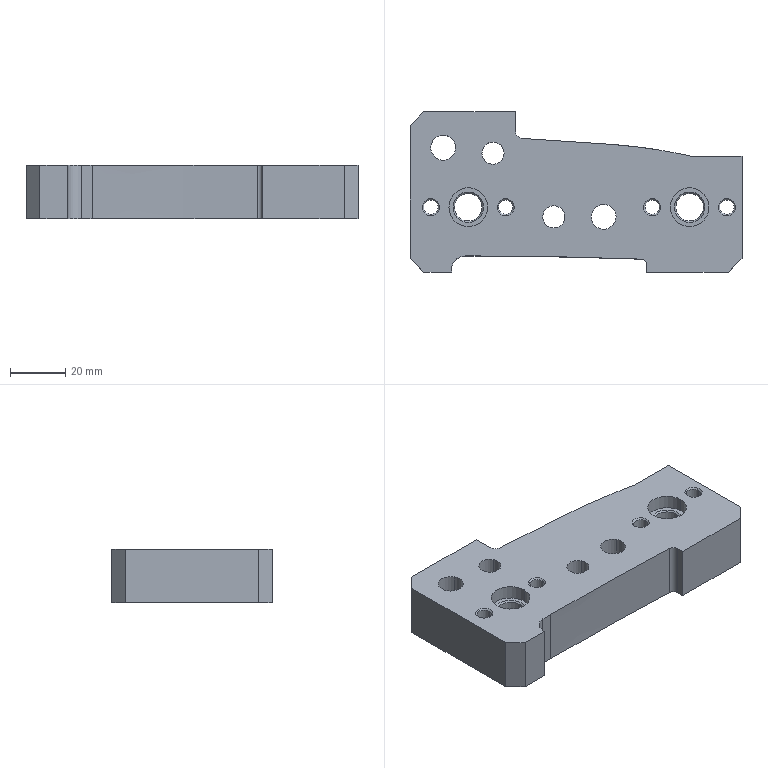Part | CATIA | 1 solid | 70 faces | box 120 x 58 x 19.5 mm | volume 94988 mm3 | cylinder 32 | plane 20 | cone 12 | other 6 | commonest cylinder face diameters 5.2 x8 10 x6 8 x4 9 x4 14 x4 15 x4